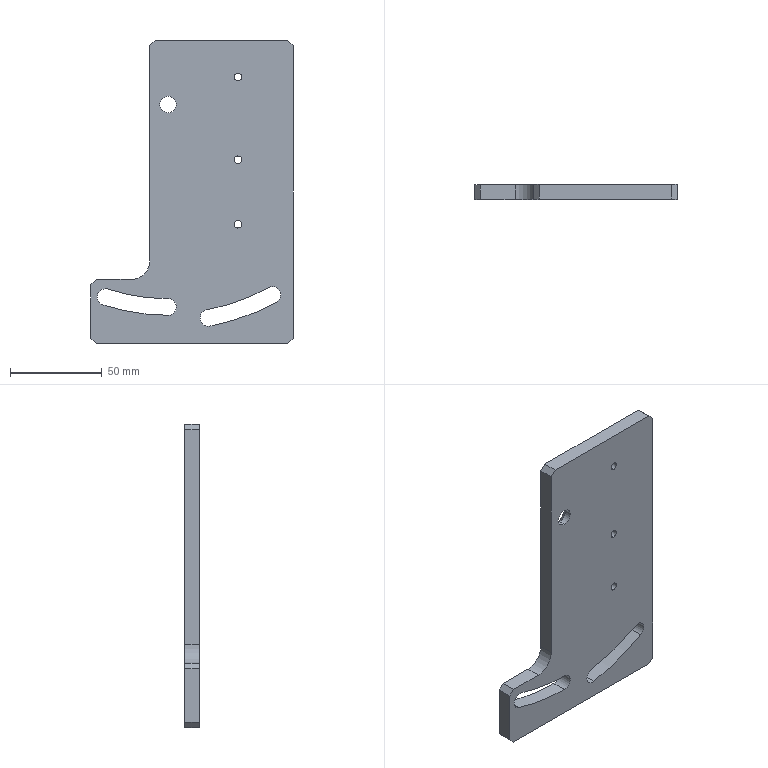Part | SolidWorks | features ICE 3, Chamfer 2, HoleWzd 2, Extrusion 1, Fillet 1 | 1 solid | 34 faces | box 110 x 8 x 165 mm | volume 104521 mm3 | cylinder 19 | plane 13 | cone 2 | commonest cylinder face diameters 9 x8 4.2 x6 20 x1 211 x1 227 x1 229 x1
STEP:
#1=CARTESIAN_POINT('',(25.,0.,60.4));
#2=VERTEX_POINT('',#1);
#3=CARTESIAN_POINT('',(25.,0.,64.6));
#4=VERTEX_POINT('',#3);
#5=CARTESIAN_POINT('',(25.,0.,62.5));
#6=DIRECTION('',(0.,1.,0.));
#7=DIRECTION('',(0.,0.,1.));
#8=AXIS2_PLACEMENT_3D('',#5,#6,#7);
#9=CIRCLE('',#8,2.1);
#10=EDGE_CURVE('',#2,#4,#9,.T.);
#11=ORIENTED_EDGE('',*,*,#10,.F.);
#12=CARTESIAN_POINT('',(25.,8.,60.4));
#13=VERTEX_POINT('',#12);
#14=CARTESIAN_POINT('',(25.,8.,60.4));
#15=DIRECTION('',(0.,1.,0.));
#16=VECTOR('',#15,1000.);
#17=LINE('',#14,#16);
#18=EDGE_CURVE('',#2,#13,#17,.T.);
#19=ORIENTED_EDGE('',*,*,#18,.T.);
#20=CARTESIAN_POINT('',(25.,8.,64.6));
#21=VERTEX_POINT('',#20);
#22=CARTESIAN_POINT('',(25.,8.,62.5));
#23=DIRECTION('',(0.,1.,0.));
#24=DIRECTION('',(0.,0.,1.));
#25=AXIS2_PLACEMENT_3D('',#22,#23,#24);
#26=CIRCLE('',#25,2.1);
#27=EDGE_CURVE('',#13,#21,#26,.T.);
#28=ORIENTED_EDGE('',*,*,#27,.T.);
#29=CARTESIAN_POINT('',(25.,8.,64.6));
#30=DIRECTION('',(0.,1.,0.));
#31=VECTOR('',#30,1000.);
#32=LINE('',#29,#31);
#33=EDGE_CURVE('',#4,#21,#32,.T.);
#34=ORIENTED_EDGE('',*,*,#33,.F.);
#35=EDGE_LOOP('',(#11,#19,#28,#34));
#36=FACE_OUTER_BOUND('',#35,.T.);
#37=CARTESIAN_POINT('',(25.,8.,62.5));
#38=DIRECTION('',(0.,1.,0.));
#39=DIRECTION('',(0.,0.,1.));
#40=AXIS2_PLACEMENT_3D('',#37,#38,#39);
#41=CYLINDRICAL_SURFACE('',#40,2.1);
#42=ADVANCED_FACE('',(#36),#41,.F.);
#43=CARTESIAN_POINT('',(25.,0.,15.4));
#44=VERTEX_POINT('',#43);
#45=CARTESIAN_POINT('',(25.,0.,19.6));
#46=VERTEX_POINT('',#45);
#47=CARTESIAN_POINT('',(25.,0.,17.5));
#48=DIRECTION('',(0.,1.,0.));
#49=DIRECTION('',(0.,0.,1.));
#50=AXIS2_PLACEMENT_3D('',#47,#48,#49);
#51=CIRCLE('',#50,2.1);
#52=EDGE_CURVE('',#44,#46,#51,.T.);
#53=ORIENTED_EDGE('',*,*,#52,.F.);
#54=CARTESIAN_POINT('',(25.,8.,15.4));
#55=VERTEX_POINT('',#54);
#56=CARTESIAN_POINT('',(25.,8.,15.4));
#57=DIRECTION('',(0.,1.,0.));
#58=VECTOR('',#57,1000.);
#59=LINE('',#56,#58);
#60=EDGE_CURVE('',#44,#55,#59,.T.);
#61=ORIENTED_EDGE('',*,*,#60,.T.);
#62=CARTESIAN_POINT('',(25.,8.,19.6));
#63=VERTEX_POINT('',#62);
#64=CARTESIAN_POINT('',(25.,8.,17.5));
#65=DIRECTION('',(0.,1.,0.));
#66=DIRECTION('',(0.,0.,1.));
#67=AXIS2_PLACEMENT_3D('',#64,#65,#66);
#68=CIRCLE('',#67,2.1);
#69=EDGE_CURVE('',#55,#63,#68,.T.);
#70=ORIENTED_EDGE('',*,*,#69,.T.);
#71=CARTESIAN_POINT('',(25.,8.,19.6));
#72=DIRECTION('',(0.,1.,0.));
#73=VECTOR('',#72,1000.);
#74=LINE('',#71,#73);
#75=EDGE_CURVE('',#46,#63,#74,.T.);
#76=ORIENTED_EDGE('',*,*,#75,.F.);
#77=EDGE_LOOP('',(#53,#61,#70,#76));
#78=FACE_OUTER_BOUND('',#77,.T.);
#79=CARTESIAN_POINT('',(25.,8.,17.5));
#80=DIRECTION('',(0.,1.,0.));
#81=DIRECTION('',(0.,0.,1.));
#82=AXIS2_PLACEMENT_3D('',#79,#80,#81);
#83=CYLINDRICAL_SURFACE('',#82,2.1);
#84=ADVANCED_FACE('',(#78),#83,.F.);
#85=CARTESIAN_POINT('',(25.,0.,-19.6));
#86=VERTEX_POINT('',#85);
#87=CARTESIAN_POINT('',(25.,0.,-15.4));
#88=VERTEX_POINT('',#87);
#89=CARTESIAN_POINT('',(25.,0.,-17.5));
#90=DIRECTION('',(0.,1.,0.));
#91=DIRECTION('',(0.,0.,1.));
#92=AXIS2_PLACEMENT_3D('',#89,#90,#91);
#93=CIRCLE('',#92,2.1);
#94=EDGE_CURVE('',#86,#88,#93,.T.);
#95=ORIENTED_EDGE('',*,*,#94,.F.);
#96=CARTESIAN_POINT('',(25.,8.,-19.6));
#97=VERTEX_POINT('',#96);
#98=CARTESIAN_POINT('',(25.,8.,-19.6));
#99=DIRECTION('',(0.,1.,0.));
#100=VECTOR('',#99,1000.);
#101=LINE('',#98,#100);
#102=EDGE_CURVE('',#86,#97,#101,.T.);
#103=ORIENTED_EDGE('',*,*,#102,.T.);
#104=CARTESIAN_POINT('',(25.,8.,-15.4));
#105=VERTEX_POINT('',#104);
#106=CARTESIAN_POINT('',(25.,8.,-17.5));
#107=DIRECTION('',(0.,1.,0.));
#108=DIRECTION('',(0.,0.,1.));
#109=AXIS2_PLACEMENT_3D('',#106,#107,#108);
#110=CIRCLE('',#109,2.1);
#111=EDGE_CURVE('',#97,#105,#110,.T.);
#112=ORIENTED_EDGE('',*,*,#111,.T.);
#113=CARTESIAN_POINT('',(25.,8.,-15.4));
#114=DIRECTION('',(0.,1.,0.));
#115=VECTOR('',#114,1000.);
#116=LINE('',#113,#115);
#117=EDGE_CURVE('',#88,#105,#116,.T.);
#118=ORIENTED_EDGE('',*,*,#117,.F.);
#119=EDGE_LOOP('',(#95,#103,#112,#118));
#120=FACE_OUTER_BOUND('',#119,.T.);
#121=CARTESIAN_POINT('',(25.,8.,-17.5));
#122=DIRECTION('',(0.,1.,0.));
#123=DIRECTION('',(0.,0.,1.));
#124=AXIS2_PLACEMENT_3D('',#121,#122,#123);
#125=CYLINDRICAL_SURFACE('',#124,2.1);
#126=ADVANCED_FACE('',(#120),#125,.F.);
#127=CARTESIAN_POINT('',(43.672,0.,-51.5));
#128=VERTEX_POINT('',#127);
#129=CARTESIAN_POINT('',(45.834,0.,-59.947));
#130=VERTEX_POINT('',#129);
#131=CARTESIAN_POINT('',(43.672,0.,-56.));
#132=DIRECTION('',(0.,1.,0.));
#133=DIRECTION('',(0.,0.,1.));
#134=AXIS2_PLACEMENT_3D('',#131,#132,#133);
#135=CIRCLE('',#134,4.5);
#136=EDGE_CURVE('',#128,#130,#135,.T.);
#137=ORIENTED_EDGE('',*,*,#136,.F.);
#138=CARTESIAN_POINT('',(43.672,8.,-51.5));
#139=VERTEX_POINT('',#138);
#140=CARTESIAN_POINT('',(43.672,0.,-51.5));
#141=DIRECTION('',(0.,1.,0.));
#142=VECTOR('',#141,1000.);
#143=LINE('',#140,#142);
#144=EDGE_CURVE('',#128,#139,#143,.T.);
#145=ORIENTED_EDGE('',*,*,#144,.T.);
#146=CARTESIAN_POINT('',(45.834,8.,-59.947));
#147=VERTEX_POINT('',#146);
#148=CARTESIAN_POINT('',(43.672,8.,-56.));
#149=DIRECTION('',(0.,1.,0.));
#150=DIRECTION('',(0.,0.,1.));
#151=AXIS2_PLACEMENT_3D('',#148,#149,#150);
#152=CIRCLE('',#151,4.5);
#153=EDGE_CURVE('',#139,#147,#152,.T.);
#154=ORIENTED_EDGE('',*,*,#153,.T.);
#155=CARTESIAN_POINT('',(45.834,0.,-59.947));
#156=DIRECTION('',(0.,1.,0.));
#157=VECTOR('',#156,1000.);
#158=LINE('',#155,#157);
#159=EDGE_CURVE('',#130,#147,#158,.T.);
#160=ORIENTED_EDGE('',*,*,#159,.F.);
#161=EDGE_LOOP('',(#137,#145,#154,#160));
#162=FACE_OUTER_BOUND('',#161,.T.);
#163=CARTESIAN_POINT('',(43.672,0.,-56.));
#164=DIRECTION('',(0.,1.,0.));
#165=DIRECTION('',(0.,0.,1.));
#166=AXIS2_PLACEMENT_3D('',#163,#164,#165);
#167=CYLINDRICAL_SURFACE('',#166,4.5);
#168=ADVANCED_FACE('',(#162),#167,.F.);
#169=CARTESIAN_POINT('',(-46.992,0.,-52.616));
#170=VERTEX_POINT('',#169);
#171=CARTESIAN_POINT('',(-45.601,0.,-52.836));
#172=VERTEX_POINT('',#171);
#173=CARTESIAN_POINT('',(-46.992,0.,-57.116));
#174=DIRECTION('',(0.,1.,0.));
#175=DIRECTION('',(0.,0.,1.));
#176=AXIS2_PLACEMENT_3D('',#173,#174,#175);
#177=CIRCLE('',#176,4.5);
#178=EDGE_CURVE('',#170,#172,#177,.T.);
#179=ORIENTED_EDGE('',*,*,#178,.F.);
#180=CARTESIAN_POINT('',(-46.992,8.,-52.616));
#181=VERTEX_POINT('',#180);
#182=CARTESIAN_POINT('',(-46.992,0.,-52.616));
#183=DIRECTION('',(0.,1.,0.));
#184=VECTOR('',#183,1000.);
#185=LINE('',#182,#184);
#186=EDGE_CURVE('',#170,#181,#185,.T.);
#187=ORIENTED_EDGE('',*,*,#186,.T.);
#188=CARTESIAN_POINT('',(-45.601,8.,-52.836));
#189=VERTEX_POINT('',#188);
#190=CARTESIAN_POINT('',(-46.992,8.,-57.116));
#191=DIRECTION('',(0.,1.,0.));
#192=DIRECTION('',(0.,0.,1.));
#193=AXIS2_PLACEMENT_3D('',#190,#191,#192);
#194=CIRCLE('',#193,4.5);
#195=EDGE_CURVE('',#181,#189,#194,.T.);
#196=ORIENTED_EDGE('',*,*,#195,.T.);
#197=CARTESIAN_POINT('',(-45.601,0.,-52.836));
#198=DIRECTION('',(0.,1.,0.));
#199=VECTOR('',#198,1000.);
#200=LINE('',#197,#199);
#201=EDGE_CURVE('',#172,#189,#200,.T.);
#202=ORIENTED_EDGE('',*,*,#201,.F.);
#203=EDGE_LOOP('',(#179,#187,#196,#202));
#204=FACE_OUTER_BOUND('',#203,.T.);
#205=CARTESIAN_POINT('',(-46.992,0.,-57.116));
#206=DIRECTION('',(0.,1.,0.));
#207=DIRECTION('',(0.,0.,1.));
#208=AXIS2_PLACEMENT_3D('',#205,#206,#207);
#209=CYLINDRICAL_SURFACE('',#208,4.5);
#210=ADVANCED_FACE('',(#204),#209,.F.);
#211=CARTESIAN_POINT('',(-13.,3.54,43.));
#212=VERTEX_POINT('',#211);
#213=CARTESIAN_POINT('',(-13.,3.54,52.));
#214=VERTEX_POINT('',#213);
#215=CARTESIAN_POINT('',(-13.,3.54,47.5));
#216=DIRECTION('',(0.,1.,0.));
#217=DIRECTION('',(0.,0.,1.));
#218=AXIS2_PLACEMENT_3D('',#215,#216,#217);
#219=CIRCLE('',#218,4.5);
#220=EDGE_CURVE('',#212,#214,#219,.T.);
#221=ORIENTED_EDGE('',*,*,#220,.F.);
#222=CARTESIAN_POINT('',(-13.,8.,38.54));
#223=VERTEX_POINT('',#222);
#224=CARTESIAN_POINT('',(-13.,8.,38.54));
#225=DIRECTION('',(0.,0.7071,-0.7071));
#226=VECTOR('',#225,1000.);
#227=LINE('',#224,#226);
#228=EDGE_CURVE('',#212,#223,#227,.T.);
#229=ORIENTED_EDGE('',*,*,#228,.T.);
#230=CARTESIAN_POINT('',(-13.,8.,56.46));
#231=VERTEX_POINT('',#230);
#232=CARTESIAN_POINT('',(-13.,8.,47.5));
#233=DIRECTION('',(0.,1.,0.));
#234=DIRECTION('',(0.,0.,1.));
#235=AXIS2_PLACEMENT_3D('',#232,#233,#234);
#236=CIRCLE('',#235,8.96);
#237=EDGE_CURVE('',#223,#231,#236,.T.);
#238=ORIENTED_EDGE('',*,*,#237,.T.);
#239=CARTESIAN_POINT('',(-13.,8.,56.46));
#240=DIRECTION('',(0.,0.7071,0.7071));
#241=VECTOR('',#240,1000.);
#242=LINE('',#239,#241);
#243=EDGE_CURVE('',#214,#231,#242,.T.);
#244=ORIENTED_EDGE('',*,*,#243,.F.);
#245=EDGE_LOOP('',(#221,#229,#238,#244));
#246=FACE_OUTER_BOUND('',#245,.T.);
#247=CARTESIAN_POINT('',(-13.,8.,47.5));
#248=DIRECTION('',(0.,1.,0.));
#249=DIRECTION('',(0.,0.,1.));
#250=AXIS2_PLACEMENT_3D('',#247,#248,#249);
#251=CONICAL_SURFACE('',#250,8.96,0.7854);
#252=ADVANCED_FACE('',(#246),#251,.F.);
#253=CARTESIAN_POINT('',(-13.,0.,43.));
#254=VERTEX_POINT('',#253);
#255=CARTESIAN_POINT('',(-13.,0.,52.));
#256=VERTEX_POINT('',#255);
#257=CARTESIAN_POINT('',(-13.,0.,47.5));
#258=DIRECTION('',(0.,1.,0.));
#259=DIRECTION('',(0.,0.,1.));
#260=AXIS2_PLACEMENT_3D('',#257,#258,#259);
#261=CIRCLE('',#260,4.5);
#262=EDGE_CURVE('',#254,#256,#261,.T.);
#263=ORIENTED_EDGE('',*,*,#262,.F.);
#264=CARTESIAN_POINT('',(-13.,8.,43.));
#265=DIRECTION('',(0.,1.,0.));
#266=VECTOR('',#265,1000.);
#267=LINE('',#264,#266);
#268=EDGE_CURVE('',#254,#212,#267,.T.);
#269=ORIENTED_EDGE('',*,*,#268,.T.);
#270=ORIENTED_EDGE('',*,*,#220,.T.);
#271=CARTESIAN_POINT('',(-13.,8.,52.));
#272=DIRECTION('',(0.,1.,0.));
#273=VECTOR('',#272,1000.);
#274=LINE('',#271,#273);
#275=EDGE_CURVE('',#256,#214,#274,.T.);
#276=ORIENTED_EDGE('',*,*,#275,.F.);
#277=EDGE_LOOP('',(#263,#269,#270,#276));
#278=FACE_OUTER_BOUND('',#277,.T.);
#279=CARTESIAN_POINT('',(-13.,8.,47.5));
#280=DIRECTION('',(0.,1.,0.));
#281=DIRECTION('',(0.,0.,1.));
#282=AXIS2_PLACEMENT_3D('',#279,#280,#281);
#283=CYLINDRICAL_SURFACE('',#282,4.5);
#284=ADVANCED_FACE('',(#278),#283,.F.);
#285=CARTESIAN_POINT('',(55.,8.,79.5));
#286=VERTEX_POINT('',#285);
#287=CARTESIAN_POINT('',(55.,8.,-79.5));
#288=VERTEX_POINT('',#287);
#289=CARTESIAN_POINT('',(55.,8.,-82.5));
#290=DIRECTION('',(0.,0.,-1.));
#291=VECTOR('',#290,1000.);
#292=LINE('',#289,#291);
#293=EDGE_CURVE('',#286,#288,#292,.T.);
#294=ORIENTED_EDGE('',*,*,#293,.F.);
#295=CARTESIAN_POINT('',(55.,0.,79.5));
#296=VERTEX_POINT('',#295);
#297=CARTESIAN_POINT('',(55.,8.,79.5));
#298=DIRECTION('',(0.,-1.,0.));
#299=VECTOR('',#298,1000.);
#300=LINE('',#297,#299);
#301=EDGE_CURVE('',#286,#296,#300,.T.);
#302=ORIENTED_EDGE('',*,*,#301,.T.);
#303=CARTESIAN_POINT('',(55.,0.,-79.5));
#304=VERTEX_POINT('',#303);
#305=CARTESIAN_POINT('',(55.,0.,-82.5));
#306=DIRECTION('',(0.,0.,-1.));
#307=VECTOR('',#306,1000.);
#308=LINE('',#305,#307);
#309=EDGE_CURVE('',#296,#304,#308,.T.);
#310=ORIENTED_EDGE('',*,*,#309,.T.);
#311=CARTESIAN_POINT('',(55.,8.,-79.5));
#312=DIRECTION('',(0.,1.,0.));
#313=VECTOR('',#312,1000.);
#314=LINE('',#311,#313);
#315=EDGE_CURVE('',#304,#288,#314,.T.);
#316=ORIENTED_EDGE('',*,*,#315,.T.);
#317=EDGE_LOOP('',(#294,#302,#310,#316));
#318=FACE_OUTER_BOUND('',#317,.T.);
#319=CARTESIAN_POINT('',(55.,8.,-82.5));
#320=DIRECTION('',(-1.,0.,0.));
#321=DIRECTION('',(0.,0.,1.));
#322=AXIS2_PLACEMENT_3D('',#319,#320,#321);
#323=PLANE('',#322);
#324=ADVANCED_FACE('',(#318),#323,.F.);
#325=CARTESIAN_POINT('',(52.,0.,-82.5));
#326=VERTEX_POINT('',#325);
#327=CARTESIAN_POINT('',(-52.,0.,-82.5));
#328=VERTEX_POINT('',#327);
#329=CARTESIAN_POINT('',(-55.,0.,-82.5));
#330=DIRECTION('',(-1.,0.,0.));
#331=VECTOR('',#330,1000.);
#332=LINE('',#329,#331);
#333=EDGE_CURVE('',#326,#328,#332,.T.);
#334=ORIENTED_EDGE('',*,*,#333,.T.);
#335=CARTESIAN_POINT('',(-52.,8.,-82.5));
#336=VERTEX_POINT('',#335);
#337=CARTESIAN_POINT('',(-52.,8.,-82.5));
#338=DIRECTION('',(0.,1.,0.));
#339=VECTOR('',#338,1000.);
#340=LINE('',#337,#339);
#341=EDGE_CURVE('',#328,#336,#340,.T.);
#342=ORIENTED_EDGE('',*,*,#341,.T.);
#343=CARTESIAN_POINT('',(52.,8.,-82.5));
#344=VERTEX_POINT('',#343);
#345=CARTESIAN_POINT('',(-55.,8.,-82.5));
#346=DIRECTION('',(-1.,0.,0.));
#347=VECTOR('',#346,1000.);
#348=LINE('',#345,#347);
#349=EDGE_CURVE('',#344,#336,#348,.T.);
#350=ORIENTED_EDGE('',*,*,#349,.F.);
#351=CARTESIAN_POINT('',(52.,8.,-82.5));
#352=DIRECTION('',(0.,-1.,0.));
#353=VECTOR('',#352,1000.);
#354=LINE('',#351,#353);
#355=EDGE_CURVE('',#344,#326,#354,.T.);
#356=ORIENTED_EDGE('',*,*,#355,.T.);
#357=EDGE_LOOP('',(#334,#342,#350,#356));
#358=FACE_OUTER_BOUND('',#357,.T.);
#359=CARTESIAN_POINT('',(-55.,8.,-82.5));
#360=DIRECTION('',(0.,0.,1.));
#361=DIRECTION('',(1.,0.,0.));
#362=AXIS2_PLACEMENT_3D('',#359,#360,#361);
#363=PLANE('',#362);
#364=ADVANCED_FACE('',(#358),#363,.F.);
#365=CARTESIAN_POINT('',(-55.,0.,-79.5));
#366=VERTEX_POINT('',#365);
#367=CARTESIAN_POINT('',(-55.,0.,-50.5));
#368=VERTEX_POINT('',#367);
#369=CARTESIAN_POINT('',(-55.,0.,-82.5));
#370=DIRECTION('',(0.,0.,1.));
#371=VECTOR('',#370,1000.);
#372=LINE('',#369,#371);
#373=EDGE_CURVE('',#366,#368,#372,.T.);
#374=ORIENTED_EDGE('',*,*,#373,.T.);
#375=CARTESIAN_POINT('',(-55.,8.,-50.5));
#376=VERTEX_POINT('',#375);
#377=CARTESIAN_POINT('',(-55.,8.,-50.5));
#378=DIRECTION('',(0.,1.,0.));
#379=VECTOR('',#378,1000.);
#380=LINE('',#377,#379);
#381=EDGE_CURVE('',#368,#376,#380,.T.);
#382=ORIENTED_EDGE('',*,*,#381,.T.);
#383=CARTESIAN_POINT('',(-55.,8.,-79.5));
#384=VERTEX_POINT('',#383);
#385=CARTESIAN_POINT('',(-55.,8.,-82.5));
#386=DIRECTION('',(0.,0.,1.));
#387=VECTOR('',#386,1000.);
#388=LINE('',#385,#387);
#389=EDGE_CURVE('',#384,#376,#388,.T.);
#390=ORIENTED_EDGE('',*,*,#389,.F.);
#391=CARTESIAN_POINT('',(-55.,8.,-79.5));
#392=DIRECTION('',(0.,-1.,0.));
#393=VECTOR('',#392,1000.);
#394=LINE('',#391,#393);
#395=EDGE_CURVE('',#384,#366,#394,.T.);
#396=ORIENTED_EDGE('',*,*,#395,.T.);
#397=EDGE_LOOP('',(#374,#382,#390,#396));
#398=FACE_OUTER_BOUND('',#397,.T.);
#399=CARTESIAN_POINT('',(-55.,8.,-82.5));
#400=DIRECTION('',(1.,0.,0.));
#401=DIRECTION('',(0.,0.,-1.));
#402=AXIS2_PLACEMENT_3D('',#399,#400,#401);
#403=PLANE('',#402);
#404=ADVANCED_FACE('',(#398),#403,.F.);
#405=CARTESIAN_POINT('',(-20.,0.,82.5));
#406=VERTEX_POINT('',#405);
#407=CARTESIAN_POINT('',(52.,0.,82.5));
#408=VERTEX_POINT('',#407);
#409=CARTESIAN_POINT('',(-55.,0.,82.5));
#410=DIRECTION('',(1.,0.,0.));
#411=VECTOR('',#410,1000.);
#412=LINE('',#409,#411);
#413=EDGE_CURVE('',#406,#408,#412,.T.);
#414=ORIENTED_EDGE('',*,*,#413,.T.);
#415=CARTESIAN_POINT('',(52.,8.,82.5));
#416=VERTEX_POINT('',#415);
#417=CARTESIAN_POINT('',(52.,8.,82.5));
#418=DIRECTION('',(0.,1.,0.));
#419=VECTOR('',#418,1000.);
#420=LINE('',#417,#419);
#421=EDGE_CURVE('',#408,#416,#420,.T.);
#422=ORIENTED_EDGE('',*,*,#421,.T.);
#423=CARTESIAN_POINT('',(-20.,8.,82.5));
#424=VERTEX_POINT('',#423);
#425=CARTESIAN_POINT('',(-55.,8.,82.5));
#426=DIRECTION('',(1.,0.,0.));
#427=VECTOR('',#426,1000.);
#428=LINE('',#425,#427);
#429=EDGE_CURVE('',#424,#416,#428,.T.);
#430=ORIENTED_EDGE('',*,*,#429,.F.);
#431=CARTESIAN_POINT('',(-20.,8.,82.5));
#432=DIRECTION('',(0.,-1.,0.));
#433=VECTOR('',#432,1000.);
#434=LINE('',#431,#433);
#435=EDGE_CURVE('',#424,#406,#434,.T.);
#436=ORIENTED_EDGE('',*,*,#435,.T.);
#437=EDGE_LOOP('',(#414,#422,#430,#436));
#438=FACE_OUTER_BOUND('',#437,.T.);
#439=CARTESIAN_POINT('',(-55.,8.,82.5));
#440=DIRECTION('',(0.,0.,-1.));
#441=DIRECTION('',(-1.,0.,0.));
#442=AXIS2_PLACEMENT_3D('',#439,#440,#441);
#443=PLANE('',#442);
#444=ADVANCED_FACE('',(#438),#443,.F.);
#445=CARTESIAN_POINT('',(25.,8.,62.5));
#446=DIRECTION('',(0.,1.,0.));
#447=DIRECTION('',(0.,0.,1.));
#448=AXIS2_PLACEMENT_3D('',#445,#446,#447);
#449=CIRCLE('',#448,2.1);
#450=EDGE_CURVE('',#21,#13,#449,.T.);
#451=ORIENTED_EDGE('',*,*,#450,.F.);
#452=ORIENTED_EDGE('',*,*,#27,.F.);
#453=EDGE_LOOP('',(#451,#452));
#454=FACE_BOUND('',#453,.T.);
#455=CARTESIAN_POINT('',(25.,8.,17.5));
#456=DIRECTION('',(0.,1.,0.));
#457=DIRECTION('',(0.,0.,1.));
#458=AXIS2_PLACEMENT_3D('',#455,#456,#457);
#459=CIRCLE('',#458,2.1);
#460=EDGE_CURVE('',#63,#55,#459,.T.);
#461=ORIENTED_EDGE('',*,*,#460,.F.);
#462=ORIENTED_EDGE('',*,*,#69,.F.);
#463=EDGE_LOOP('',(#461,#462));
#464=FACE_BOUND('',#463,.T.);
#465=CARTESIAN_POINT('',(25.,8.,-17.5));
#466=DIRECTION('',(0.,1.,0.));
#467=DIRECTION('',(0.,0.,1.));
#468=AXIS2_PLACEMENT_3D('',#465,#466,#467);
#469=CIRCLE('',#468,2.1);
#470=EDGE_CURVE('',#105,#97,#469,.T.);
#471=ORIENTED_EDGE('',*,*,#470,.F.);
#472=ORIENTED_EDGE('',*,*,#111,.F.);
#473=EDGE_LOOP('',(#471,#472));
#474=FACE_BOUND('',#473,.T.);
#475=CARTESIAN_POINT('',(41.511,8.,-52.053));
#476=VERTEX_POINT('',#475);
#477=CARTESIAN_POINT('',(43.672,8.,-56.));
#478=DIRECTION('',(0.,1.,0.));
#479=DIRECTION('',(0.,0.,1.));
#480=AXIS2_PLACEMENT_3D('',#477,#478,#479);
#481=CIRCLE('',#480,4.5);
#482=EDGE_CURVE('',#476,#139,#481,.T.);
#483=ORIENTED_EDGE('',*,*,#482,.F.);
#484=CARTESIAN_POINT('',(8.08,8.,-64.025));
#485=VERTEX_POINT('',#484);
#486=CARTESIAN_POINT('',(-13.,8.,47.5));
#487=DIRECTION('',(0.,-1.,0.));
#488=DIRECTION('',(0.,0.,1.));
#489=AXIS2_PLACEMENT_3D('',#486,#487,#488);
#490=CIRCLE('',#489,113.5);
#491=EDGE_CURVE('',#485,#476,#490,.T.);
#492=ORIENTED_EDGE('',*,*,#491,.F.);
#493=CARTESIAN_POINT('',(9.751,8.,-72.869));
#494=VERTEX_POINT('',#493);
#495=CARTESIAN_POINT('',(8.915,8.,-68.447));
#496=DIRECTION('',(0.,1.,0.));
#497=DIRECTION('',(0.,0.,1.));
#498=AXIS2_PLACEMENT_3D('',#495,#496,#497);
#499=CIRCLE('',#498,4.5);
#500=EDGE_CURVE('',#494,#485,#499,.T.);
#501=ORIENTED_EDGE('',*,*,#500,.F.);
#502=CARTESIAN_POINT('',(-13.,8.,47.5));
#503=DIRECTION('',(0.,1.,0.));
#504=DIRECTION('',(0.,0.,1.));
#505=AXIS2_PLACEMENT_3D('',#502,#503,#504);
#506=CIRCLE('',#505,122.5);
#507=EDGE_CURVE('',#147,#494,#506,.T.);
#508=ORIENTED_EDGE('',*,*,#507,.F.);
#509=ORIENTED_EDGE('',*,*,#153,.F.);
#510=EDGE_LOOP('',(#483,#492,#501,#508,#509));
#511=FACE_BOUND('',#510,.T.);
#512=CARTESIAN_POINT('',(-13.,8.,-58.));
#513=VERTEX_POINT('',#512);
#514=CARTESIAN_POINT('',(-13.,8.,-67.));
#515=VERTEX_POINT('',#514);
#516=CARTESIAN_POINT('',(-13.,8.,-62.5));
#517=DIRECTION('',(0.,1.,0.));
#518=DIRECTION('',(0.,0.,1.));
#519=AXIS2_PLACEMENT_3D('',#516,#517,#518);
#520=CIRCLE('',#519,4.5);
#521=EDGE_CURVE('',#513,#515,#520,.T.);
#522=ORIENTED_EDGE('',*,*,#521,.F.);
#523=CARTESIAN_POINT('',(-13.,8.,47.5));
#524=DIRECTION('',(0.,1.,0.));
#525=DIRECTION('',(0.,0.,1.));
#526=AXIS2_PLACEMENT_3D('',#523,#524,#525);
#527=CIRCLE('',#526,105.5);
#528=EDGE_CURVE('',#513,#189,#527,.T.);
#529=ORIENTED_EDGE('',*,*,#528,.T.);
#530=ORIENTED_EDGE('',*,*,#195,.F.);
#531=CARTESIAN_POINT('',(-48.382,8.,-61.396));
#532=VERTEX_POINT('',#531);
#533=CARTESIAN_POINT('',(-46.992,8.,-57.116));
#534=DIRECTION('',(0.,1.,0.));
#535=DIRECTION('',(0.,0.,1.));
#536=AXIS2_PLACEMENT_3D('',#533,#534,#535);
#537=CIRCLE('',#536,4.5);
#538=EDGE_CURVE('',#532,#181,#537,.T.);
#539=ORIENTED_EDGE('',*,*,#538,.F.);
#540=CARTESIAN_POINT('',(-13.,8.,47.5));
#541=DIRECTION('',(0.,1.,0.));
#542=DIRECTION('',(0.,0.,1.));
#543=AXIS2_PLACEMENT_3D('',#540,#541,#542);
#544=CIRCLE('',#543,114.5);
#545=EDGE_CURVE('',#515,#532,#544,.T.);
#546=ORIENTED_EDGE('',*,*,#545,.F.);
#547=EDGE_LOOP('',(#522,#529,#530,#539,#546));
#548=FACE_BOUND('',#547,.T.);
#549=CARTESIAN_POINT('',(-13.,8.,47.5));
#550=DIRECTION('',(0.,1.,0.));
#551=DIRECTION('',(0.,0.,1.));
#552=AXIS2_PLACEMENT_3D('',#549,#550,#551);
#553=CIRCLE('',#552,8.96);
#554=EDGE_CURVE('',#231,#223,#553,.T.);
#555=ORIENTED_EDGE('',*,*,#554,.F.);
#556=ORIENTED_EDGE('',*,*,#237,.F.);
#557=EDGE_LOOP('',(#555,#556));
#558=FACE_BOUND('',#557,.T.);
#559=ORIENTED_EDGE('',*,*,#429,.T.);
#560=CARTESIAN_POINT('',(67.25,8.,67.25));
#561=DIRECTION('',(0.7071,0.,-0.7071));
#562=VECTOR('',#561,1000.);
#563=LINE('',#560,#562);
#564=EDGE_CURVE('',#416,#286,#563,.T.);
#565=ORIENTED_EDGE('',*,*,#564,.T.);
#566=ORIENTED_EDGE('',*,*,#293,.T.);
#567=CARTESIAN_POINT('',(67.25,8.,-67.25));
#568=DIRECTION('',(-0.7071,0.,-0.7071));
#569=VECTOR('',#568,1000.);
#570=LINE('',#567,#569);
#571=EDGE_CURVE('',#288,#344,#570,.T.);
#572=ORIENTED_EDGE('',*,*,#571,.T.);
#573=ORIENTED_EDGE('',*,*,#349,.T.);
#574=CARTESIAN_POINT('',(-67.25,8.,-67.25));
#575=DIRECTION('',(-0.7071,0.,0.7071));
#576=VECTOR('',#575,1000.);
#577=LINE('',#574,#576);
#578=EDGE_CURVE('',#336,#384,#577,.T.);
#579=ORIENTED_EDGE('',*,*,#578,.T.);
#580=ORIENTED_EDGE('',*,*,#389,.T.);
#581=CARTESIAN_POINT('',(-52.,8.,-47.5));
#582=VERTEX_POINT('',#581);
#583=CARTESIAN_POINT('',(-2.25,8.,2.25));
#584=DIRECTION('',(0.7071,0.,0.7071));
#585=VECTOR('',#584,1000.);
#586=LINE('',#583,#585);
#587=EDGE_CURVE('',#376,#582,#586,.T.);
#588=ORIENTED_EDGE('',*,*,#587,.T.);
#589=CARTESIAN_POINT('',(-33.,8.,-47.5));
#590=VERTEX_POINT('',#589);
#591=CARTESIAN_POINT('',(-55.,8.,-47.5));
#592=DIRECTION('',(-1.,0.,0.));
#593=VECTOR('',#592,1000.);
#594=LINE('',#591,#593);
#595=EDGE_CURVE('',#590,#582,#594,.T.);
#596=ORIENTED_EDGE('',*,*,#595,.F.);
#597=CARTESIAN_POINT('',(-23.,8.,-37.5));
#598=VERTEX_POINT('',#597);
#599=CARTESIAN_POINT('',(-33.,8.,-37.5));
#600=DIRECTION('',(0.,-1.,0.));
#601=DIRECTION('',(0.,0.,1.));
#602=AXIS2_PLACEMENT_3D('',#599,#600,#601);
#603=CIRCLE('',#602,10.);
#604=EDGE_CURVE('',#590,#598,#603,.T.);
#605=ORIENTED_EDGE('',*,*,#604,.T.);
#606=CARTESIAN_POINT('',(-23.,8.,79.5));
#607=VERTEX_POINT('',#606);
#608=CARTESIAN_POINT('',(-23.,8.,82.5));
#609=DIRECTION('',(0.,0.,-1.));
#610=VECTOR('',#609,1000.);
#611=LINE('',#608,#610);
#612=EDGE_CURVE('',#607,#598,#611,.T.);
#613=ORIENTED_EDGE('',*,*,#612,.F.);
#614=CARTESIAN_POINT('',(-51.25,8.,51.25));
#615=DIRECTION('',(0.7071,0.,0.7071));
#616=VECTOR('',#615,1000.);
#617=LINE('',#614,#616);
#618=EDGE_CURVE('',#607,#424,#617,.T.);
#619=ORIENTED_EDGE('',*,*,#618,.T.);
#620=EDGE_LOOP('',(#559,#565,#566,#572,#573,#579,#580,#588,#596,#605,#613,#619));
#621=FACE_OUTER_BOUND('',#620,.T.);
#622=CARTESIAN_POINT('',(0.,8.,0.));
#623=DIRECTION('',(0.,1.,0.));
#624=DIRECTION('',(0.,0.,1.));
#625=AXIS2_PLACEMENT_3D('',#622,#623,#624);
#626=PLANE('',#625);
#627=ADVANCED_FACE('',(#454,#464,#474,#511,#548,#558,#621),#626,.T.);
#628=CARTESIAN_POINT('',(25.,0.,62.5));
#629=DIRECTION('',(0.,1.,0.));
#630=DIRECTION('',(0.,0.,1.));
#631=AXIS2_PLACEMENT_3D('',#628,#629,#630);
#632=CIRCLE('',#631,2.1);
#633=EDGE_CURVE('',#4,#2,#632,.T.);
#634=ORIENTED_EDGE('',*,*,#633,.T.);
#635=ORIENTED_EDGE('',*,*,#10,.T.);
#636=EDGE_LOOP('',(#634,#635));
#637=FACE_BOUND('',#636,.T.);
#638=CARTESIAN_POINT('',(25.,0.,17.5));
#639=DIRECTION('',(0.,1.,0.));
#640=DIRECTION('',(0.,0.,1.));
#641=AXIS2_PLACEMENT_3D('',#638,#639,#640);
#642=CIRCLE('',#641,2.1);
#643=EDGE_CURVE('',#46,#44,#642,.T.);
#644=ORIENTED_EDGE('',*,*,#643,.T.);
#645=ORIENTED_EDGE('',*,*,#52,.T.);
#646=EDGE_LOOP('',(#644,#645));
#647=FACE_BOUND('',#646,.T.);
#648=CARTESIAN_POINT('',(25.,0.,-17.5));
#649=DIRECTION('',(0.,1.,0.));
#650=DIRECTION('',(0.,0.,1.));
#651=AXIS2_PLACEMENT_3D('',#648,#649,#650);
#652=CIRCLE('',#651,2.1);
#653=EDGE_CURVE('',#88,#86,#652,.T.);
#654=ORIENTED_EDGE('',*,*,#653,.T.);
#655=ORIENTED_EDGE('',*,*,#94,.T.);
#656=EDGE_LOOP('',(#654,#655));
#657=FACE_BOUND('',#656,.T.);
#658=CARTESIAN_POINT('',(8.08,0.,-64.025));
#659=VERTEX_POINT('',#658);
#660=CARTESIAN_POINT('',(41.511,0.,-52.053));
#661=VERTEX_POINT('',#660);
#662=CARTESIAN_POINT('',(-13.,0.,47.5));
#663=DIRECTION('',(0.,-1.,0.));
#664=DIRECTION('',(0.,0.,1.));
#665=AXIS2_PLACEMENT_3D('',#662,#663,#664);
#666=CIRCLE('',#665,113.5);
#667=EDGE_CURVE('',#659,#661,#666,.T.);
#668=ORIENTED_EDGE('',*,*,#667,.T.);
#669=CARTESIAN_POINT('',(43.672,0.,-56.));
#670=DIRECTION('',(0.,1.,0.));
#671=DIRECTION('',(0.,0.,1.));
#672=AXIS2_PLACEMENT_3D('',#669,#670,#671);
#673=CIRCLE('',#672,4.5);
#674=EDGE_CURVE('',#661,#128,#673,.T.);
#675=ORIENTED_EDGE('',*,*,#674,.T.);
#676=ORIENTED_EDGE('',*,*,#136,.T.);
#677=CARTESIAN_POINT('',(9.751,0.,-72.869));
#678=VERTEX_POINT('',#677);
#679=CARTESIAN_POINT('',(-13.,0.,47.5));
#680=DIRECTION('',(0.,1.,0.));
#681=DIRECTION('',(0.,0.,1.));
#682=AXIS2_PLACEMENT_3D('',#679,#680,#681);
#683=CIRCLE('',#682,122.5);
#684=EDGE_CURVE('',#130,#678,#683,.T.);
#685=ORIENTED_EDGE('',*,*,#684,.T.);
#686=CARTESIAN_POINT('',(8.915,0.,-68.447));
#687=DIRECTION('',(0.,1.,0.));
#688=DIRECTION('',(0.,0.,1.));
#689=AXIS2_PLACEMENT_3D('',#686,#687,#688);
#690=CIRCLE('',#689,4.5);
#691=EDGE_CURVE('',#678,#659,#690,.T.);
#692=ORIENTED_EDGE('',*,*,#691,.T.);
#693=EDGE_LOOP('',(#668,#675,#676,#685,#692));
#694=FACE_BOUND('',#693,.T.);
#695=CARTESIAN_POINT('',(-13.,0.,-58.));
#696=VERTEX_POINT('',#695);
#697=CARTESIAN_POINT('',(-13.,0.,47.5));
#698=DIRECTION('',(0.,1.,0.));
#699=DIRECTION('',(0.,0.,1.));
#700=AXIS2_PLACEMENT_3D('',#697,#698,#699);
#701=CIRCLE('',#700,105.5);
#702=EDGE_CURVE('',#696,#172,#701,.T.);
#703=ORIENTED_EDGE('',*,*,#702,.F.);
#704=CARTESIAN_POINT('',(-13.,0.,-67.));
#705=VERTEX_POINT('',#704);
#706=CARTESIAN_POINT('',(-13.,0.,-62.5));
#707=DIRECTION('',(0.,1.,0.));
#708=DIRECTION('',(0.,0.,1.));
#709=AXIS2_PLACEMENT_3D('',#706,#707,#708);
#710=CIRCLE('',#709,4.5);
#711=EDGE_CURVE('',#696,#705,#710,.T.);
#712=ORIENTED_EDGE('',*,*,#711,.T.);
#713=CARTESIAN_POINT('',(-48.382,0.,-61.396));
#714=VERTEX_POINT('',#713);
#715=CARTESIAN_POINT('',(-13.,0.,47.5));
#716=DIRECTION('',(0.,1.,0.));
#717=DIRECTION('',(0.,0.,1.));
#718=AXIS2_PLACEMENT_3D('',#715,#716,#717);
#719=CIRCLE('',#718,114.5);
#720=EDGE_CURVE('',#705,#714,#719,.T.);
#721=ORIENTED_EDGE('',*,*,#720,.T.);
#722=CARTESIAN_POINT('',(-46.992,0.,-57.116));
#723=DIRECTION('',(0.,1.,0.));
#724=DIRECTION('',(0.,0.,1.));
#725=AXIS2_PLACEMENT_3D('',#722,#723,#724);
#726=CIRCLE('',#725,4.5);
#727=EDGE_CURVE('',#714,#170,#726,.T.);
#728=ORIENTED_EDGE('',*,*,#727,.T.);
#729=ORIENTED_EDGE('',*,*,#178,.T.);
#730=EDGE_LOOP('',(#703,#712,#721,#728,#729));
#731=FACE_BOUND('',#730,.T.);
#732=CARTESIAN_POINT('',(-13.,0.,47.5));
#733=DIRECTION('',(0.,1.,0.));
#734=DIRECTION('',(0.,0.,1.));
#735=AXIS2_PLACEMENT_3D('',#732,#733,#734);
#736=CIRCLE('',#735,4.5);
#737=EDGE_CURVE('',#256,#254,#736,.T.);
#738=ORIENTED_EDGE('',*,*,#737,.T.);
#739=ORIENTED_EDGE('',*,*,#262,.T.);
#740=EDGE_LOOP('',(#738,#739));
#741=FACE_BOUND('',#740,.T.);
#742=ORIENTED_EDGE('',*,*,#309,.F.);
#743=CARTESIAN_POINT('',(55.,0.,79.5));
#744=DIRECTION('',(-0.7071,0.,0.7071));
#745=VECTOR('',#744,1000.);
#746=LINE('',#743,#745);
#747=EDGE_CURVE('',#296,#408,#746,.T.);
#748=ORIENTED_EDGE('',*,*,#747,.T.);
#749=ORIENTED_EDGE('',*,*,#413,.F.);
#750=CARTESIAN_POINT('',(-23.,0.,79.5));
#751=VERTEX_POINT('',#750);
#752=CARTESIAN_POINT('',(-23.,0.,79.5));
#753=DIRECTION('',(-0.7071,0.,-0.7071));
#754=VECTOR('',#753,1000.);
#755=LINE('',#752,#754);
#756=EDGE_CURVE('',#406,#751,#755,.T.);
#757=ORIENTED_EDGE('',*,*,#756,.T.);
#758=CARTESIAN_POINT('',(-23.,0.,-37.5));
#759=VERTEX_POINT('',#758);
#760=CARTESIAN_POINT('',(-23.,0.,82.5));
#761=DIRECTION('',(0.,0.,-1.));
#762=VECTOR('',#761,1000.);
#763=LINE('',#760,#762);
#764=EDGE_CURVE('',#751,#759,#763,.T.);
#765=ORIENTED_EDGE('',*,*,#764,.T.);
#766=CARTESIAN_POINT('',(-33.,0.,-47.5));
#767=VERTEX_POINT('',#766);
#768=CARTESIAN_POINT('',(-33.,0.,-37.5));
#769=DIRECTION('',(0.,1.,0.));
#770=DIRECTION('',(0.,0.,1.));
#771=AXIS2_PLACEMENT_3D('',#768,#769,#770);
#772=CIRCLE('',#771,10.);
#773=EDGE_CURVE('',#759,#767,#772,.T.);
#774=ORIENTED_EDGE('',*,*,#773,.T.);
#775=CARTESIAN_POINT('',(-52.,0.,-47.5));
#776=VERTEX_POINT('',#775);
#777=CARTESIAN_POINT('',(-55.,0.,-47.5));
#778=DIRECTION('',(-1.,0.,0.));
#779=VECTOR('',#778,1000.);
#780=LINE('',#777,#779);
#781=EDGE_CURVE('',#767,#776,#780,.T.);
#782=ORIENTED_EDGE('',*,*,#781,.T.);
#783=CARTESIAN_POINT('',(-55.,0.,-50.5));
#784=DIRECTION('',(-0.7071,0.,-0.7071));
#785=VECTOR('',#784,1000.);
#786=LINE('',#783,#785);
#787=EDGE_CURVE('',#776,#368,#786,.T.);
#788=ORIENTED_EDGE('',*,*,#787,.T.);
#789=ORIENTED_EDGE('',*,*,#373,.F.);
#790=CARTESIAN_POINT('',(-55.,0.,-79.5));
#791=DIRECTION('',(0.7071,0.,-0.7071));
#792=VECTOR('',#791,1000.);
#793=LINE('',#790,#792);
#794=EDGE_CURVE('',#366,#328,#793,.T.);
#795=ORIENTED_EDGE('',*,*,#794,.T.);
#796=ORIENTED_EDGE('',*,*,#333,.F.);
#797=CARTESIAN_POINT('',(52.,0.,-82.5));
#798=DIRECTION('',(0.7071,0.,0.7071));
#799=VECTOR('',#798,1000.);
#800=LINE('',#797,#799);
#801=EDGE_CURVE('',#326,#304,#800,.T.);
#802=ORIENTED_EDGE('',*,*,#801,.T.);
#803=EDGE_LOOP('',(#742,#748,#749,#757,#765,#774,#782,#788,#789,#795,#796,#802));
#804=FACE_OUTER_BOUND('',#803,.T.);
#805=CARTESIAN_POINT('',(0.,0.,0.));
#806=DIRECTION('',(0.,1.,0.));
#807=DIRECTION('',(0.,0.,1.));
#808=AXIS2_PLACEMENT_3D('',#805,#806,#807);
#809=PLANE('',#808);
#810=ADVANCED_FACE('',(#637,#647,#657,#694,#731,#741,#804),#809,.F.);
#811=ORIENTED_EDGE('',*,*,#781,.F.);
#812=CARTESIAN_POINT('',(-33.,8.,-47.5));
#813=DIRECTION('',(0.,1.,0.));
#814=VECTOR('',#813,1000.);
#815=LINE('',#812,#814);
#816=EDGE_CURVE('',#767,#590,#815,.T.);
#817=ORIENTED_EDGE('',*,*,#816,.T.);
#818=ORIENTED_EDGE('',*,*,#595,.T.);
#819=CARTESIAN_POINT('',(-52.,0.,-47.5));
#820=DIRECTION('',(0.,-1.,0.));
#821=VECTOR('',#820,1000.);
#822=LINE('',#819,#821);
#823=EDGE_CURVE('',#582,#776,#822,.T.);
#824=ORIENTED_EDGE('',*,*,#823,.T.);
#825=EDGE_LOOP('',(#811,#817,#818,#824));
#826=FACE_OUTER_BOUND('',#825,.T.);
#827=CARTESIAN_POINT('',(-55.,0.,-47.5));
#828=DIRECTION('',(0.,0.,-1.));
#829=DIRECTION('',(-1.,0.,0.));
#830=AXIS2_PLACEMENT_3D('',#827,#828,#829);
#831=PLANE('',#830);
#832=ADVANCED_FACE('',(#826),#831,.F.);
#833=ORIENTED_EDGE('',*,*,#612,.T.);
#834=CARTESIAN_POINT('',(-23.,0.,-37.5));
#835=DIRECTION('',(0.,-1.,0.));
#836=VECTOR('',#835,1000.);
#837=LINE('',#834,#836);
#838=EDGE_CURVE('',#598,#759,#837,.T.);
#839=ORIENTED_EDGE('',*,*,#838,.T.);
#840=ORIENTED_EDGE('',*,*,#764,.F.);
#841=CARTESIAN_POINT('',(-23.,0.,79.5));
#842=DIRECTION('',(0.,1.,0.));
#843=VECTOR('',#842,1000.);
#844=LINE('',#841,#843);
#845=EDGE_CURVE('',#751,#607,#844,.T.);
#846=ORIENTED_EDGE('',*,*,#845,.T.);
#847=EDGE_LOOP('',(#833,#839,#840,#846));
#848=FACE_OUTER_BOUND('',#847,.T.);
#849=CARTESIAN_POINT('',(-23.,0.,82.5));
#850=DIRECTION('',(1.,0.,0.));
#851=DIRECTION('',(0.,0.,-1.));
#852=AXIS2_PLACEMENT_3D('',#849,#850,#851);
#853=PLANE('',#852);
#854=ADVANCED_FACE('',(#848),#853,.F.);
#855=ORIENTED_EDGE('',*,*,#268,.F.);
#856=ORIENTED_EDGE('',*,*,#737,.F.);
#857=ORIENTED_EDGE('',*,*,#275,.T.);
#858=CARTESIAN_POINT('',(-13.,3.54,47.5));
#859=DIRECTION('',(0.,1.,0.));
#860=DIRECTION('',(0.,0.,1.));
#861=AXIS2_PLACEMENT_3D('',#858,#859,#860);
#862=CIRCLE('',#861,4.5);
#863=EDGE_CURVE('',#214,#212,#862,.T.);
#864=ORIENTED_EDGE('',*,*,#863,.T.);
#865=EDGE_LOOP('',(#855,#856,#857,#864));
#866=FACE_OUTER_BOUND('',#865,.T.);
#867=CARTESIAN_POINT('',(-13.,8.,47.5));
#868=DIRECTION('',(0.,1.,0.));
#869=DIRECTION('',(0.,0.,1.));
#870=AXIS2_PLACEMENT_3D('',#867,#868,#869);
#871=CYLINDRICAL_SURFACE('',#870,4.5);
#872=ADVANCED_FACE('',(#866),#871,.F.);
#873=ORIENTED_EDGE('',*,*,#228,.F.);
#874=ORIENTED_EDGE('',*,*,#863,.F.);
#875=ORIENTED_EDGE('',*,*,#243,.T.);
#876=ORIENTED_EDGE('',*,*,#554,.T.);
#877=EDGE_LOOP('',(#873,#874,#875,#876));
#878=FACE_OUTER_BOUND('',#877,.T.);
#879=CARTESIAN_POINT('',(-13.,8.,47.5));
#880=DIRECTION('',(0.,1.,0.));
#881=DIRECTION('',(0.,0.,1.));
#882=AXIS2_PLACEMENT_3D('',#879,#880,#881);
#883=CONICAL_SURFACE('',#882,8.96,0.7854);
#884=ADVANCED_FACE('',(#878),#883,.F.);
#885=ORIENTED_EDGE('',*,*,#521,.T.);
#886=CARTESIAN_POINT('',(-13.,0.,-67.));
#887=DIRECTION('',(0.,1.,0.));
#888=VECTOR('',#887,1000.);
#889=LINE('',#886,#888);
#890=EDGE_CURVE('',#705,#515,#889,.T.);
#891=ORIENTED_EDGE('',*,*,#890,.F.);
#892=ORIENTED_EDGE('',*,*,#711,.F.);
#893=CARTESIAN_POINT('',(-13.,0.,-58.));
#894=DIRECTION('',(0.,1.,0.));
#895=VECTOR('',#894,1000.);
#896=LINE('',#893,#895);
#897=EDGE_CURVE('',#696,#513,#896,.T.);
#898=ORIENTED_EDGE('',*,*,#897,.T.);
#899=EDGE_LOOP('',(#885,#891,#892,#898));
#900=FACE_OUTER_BOUND('',#899,.T.);
#901=CARTESIAN_POINT('',(-13.,0.,-62.5));
#902=DIRECTION('',(0.,1.,0.));
#903=DIRECTION('',(0.,0.,1.));
#904=AXIS2_PLACEMENT_3D('',#901,#902,#903);
#905=CYLINDRICAL_SURFACE('',#904,4.5);
#906=ADVANCED_FACE('',(#900),#905,.F.);
#907=ORIENTED_EDGE('',*,*,#528,.F.);
#908=ORIENTED_EDGE('',*,*,#897,.F.);
#909=ORIENTED_EDGE('',*,*,#702,.T.);
#910=ORIENTED_EDGE('',*,*,#201,.T.);
#911=EDGE_LOOP('',(#907,#908,#909,#910));
#912=FACE_OUTER_BOUND('',#911,.T.);
#913=CARTESIAN_POINT('',(-13.,0.,47.5));
#914=DIRECTION('',(0.,1.,0.));
#915=DIRECTION('',(0.,0.,1.));
#916=AXIS2_PLACEMENT_3D('',#913,#914,#915);
#917=CYLINDRICAL_SURFACE('',#916,105.5);
#918=ADVANCED_FACE('',(#912),#917,.T.);
#919=ORIENTED_EDGE('',*,*,#186,.F.);
#920=ORIENTED_EDGE('',*,*,#727,.F.);
#921=CARTESIAN_POINT('',(-48.382,0.,-61.396));
#922=DIRECTION('',(0.,1.,0.));
#923=VECTOR('',#922,1000.);
#924=LINE('',#921,#923);
#925=EDGE_CURVE('',#714,#532,#924,.T.);
#926=ORIENTED_EDGE('',*,*,#925,.T.);
#927=ORIENTED_EDGE('',*,*,#538,.T.);
#928=EDGE_LOOP('',(#919,#920,#926,#927));
#929=FACE_OUTER_BOUND('',#928,.T.);
#930=CARTESIAN_POINT('',(-46.992,0.,-57.116));
#931=DIRECTION('',(0.,1.,0.));
#932=DIRECTION('',(0.,0.,1.));
#933=AXIS2_PLACEMENT_3D('',#930,#931,#932);
#934=CYLINDRICAL_SURFACE('',#933,4.5);
#935=ADVANCED_FACE('',(#929),#934,.F.);
#936=ORIENTED_EDGE('',*,*,#545,.T.);
#937=ORIENTED_EDGE('',*,*,#925,.F.);
#938=ORIENTED_EDGE('',*,*,#720,.F.);
#939=ORIENTED_EDGE('',*,*,#890,.T.);
#940=EDGE_LOOP('',(#936,#937,#938,#939));
#941=FACE_OUTER_BOUND('',#940,.T.);
#942=CARTESIAN_POINT('',(-13.,0.,47.5));
#943=DIRECTION('',(0.,1.,0.));
#944=DIRECTION('',(0.,0.,1.));
#945=AXIS2_PLACEMENT_3D('',#942,#943,#944);
#946=CYLINDRICAL_SURFACE('',#945,114.5);
#947=ADVANCED_FACE('',(#941),#946,.F.);
#948=ORIENTED_EDGE('',*,*,#144,.F.);
#949=ORIENTED_EDGE('',*,*,#674,.F.);
#950=CARTESIAN_POINT('',(41.511,0.,-52.053));
#951=DIRECTION('',(0.,1.,0.));
#952=VECTOR('',#951,1000.);
#953=LINE('',#950,#952);
#954=EDGE_CURVE('',#661,#476,#953,.T.);
#955=ORIENTED_EDGE('',*,*,#954,.T.);
#956=ORIENTED_EDGE('',*,*,#482,.T.);
#957=EDGE_LOOP('',(#948,#949,#955,#956));
#958=FACE_OUTER_BOUND('',#957,.T.);
#959=CARTESIAN_POINT('',(43.672,0.,-56.));
#960=DIRECTION('',(0.,1.,0.));
#961=DIRECTION('',(0.,0.,1.));
#962=AXIS2_PLACEMENT_3D('',#959,#960,#961);
#963=CYLINDRICAL_SURFACE('',#962,4.5);
#964=ADVANCED_FACE('',(#958),#963,.F.);
#965=ORIENTED_EDGE('',*,*,#491,.T.);
#966=ORIENTED_EDGE('',*,*,#954,.F.);
#967=ORIENTED_EDGE('',*,*,#667,.F.);
#968=CARTESIAN_POINT('',(8.08,0.,-64.025));
#969=DIRECTION('',(0.,1.,0.));
#970=VECTOR('',#969,1000.);
#971=LINE('',#968,#970);
#972=EDGE_CURVE('',#659,#485,#971,.T.);
#973=ORIENTED_EDGE('',*,*,#972,.T.);
#974=EDGE_LOOP('',(#965,#966,#967,#973));
#975=FACE_OUTER_BOUND('',#974,.T.);
#976=CARTESIAN_POINT('',(-13.,0.,47.5));
#977=DIRECTION('',(0.,1.,0.));
#978=DIRECTION('',(0.,0.,1.));
#979=AXIS2_PLACEMENT_3D('',#976,#977,#978);
#980=CYLINDRICAL_SURFACE('',#979,113.5);
#981=ADVANCED_FACE('',(#975),#980,.T.);
#982=ORIENTED_EDGE('',*,*,#500,.T.);
#983=ORIENTED_EDGE('',*,*,#972,.F.);
#984=ORIENTED_EDGE('',*,*,#691,.F.);
#985=CARTESIAN_POINT('',(9.751,0.,-72.869));
#986=DIRECTION('',(0.,1.,0.));
#987=VECTOR('',#986,1000.);
#988=LINE('',#985,#987);
#989=EDGE_CURVE('',#678,#494,#988,.T.);
#990=ORIENTED_EDGE('',*,*,#989,.T.);
#991=EDGE_LOOP('',(#982,#983,#984,#990));
#992=FACE_OUTER_BOUND('',#991,.T.);
#993=CARTESIAN_POINT('',(8.915,0.,-68.447));
#994=DIRECTION('',(0.,1.,0.));
#995=DIRECTION('',(0.,0.,1.));
#996=AXIS2_PLACEMENT_3D('',#993,#994,#995);
#997=CYLINDRICAL_SURFACE('',#996,4.5);
#998=ADVANCED_FACE('',(#992),#997,.F.);
#999=ORIENTED_EDGE('',*,*,#507,.T.);
#1000=ORIENTED_EDGE('',*,*,#989,.F.);
#1001=ORIENTED_EDGE('',*,*,#684,.F.);
#1002=ORIENTED_EDGE('',*,*,#159,.T.);
#1003=EDGE_LOOP('',(#999,#1000,#1001,#1002));
#1004=FACE_OUTER_BOUND('',#1003,.T.);
#1005=CARTESIAN_POINT('',(-13.,0.,47.5));
#1006=DIRECTION('',(0.,1.,0.));
#1007=DIRECTION('',(0.,0.,1.));
#1008=AXIS2_PLACEMENT_3D('',#1005,#1006,#1007);
#1009=CYLINDRICAL_SURFACE('',#1008,122.5);
#1010=ADVANCED_FACE('',(#1004),#1009,.F.);
#1011=ORIENTED_EDGE('',*,*,#564,.F.);
#1012=ORIENTED_EDGE('',*,*,#421,.F.);
#1013=ORIENTED_EDGE('',*,*,#747,.F.);
#1014=ORIENTED_EDGE('',*,*,#301,.F.);
#1015=EDGE_LOOP('',(#1011,#1012,#1013,#1014));
#1016=FACE_OUTER_BOUND('',#1015,.T.);
#1017=CARTESIAN_POINT('',(55.,8.,79.5));
#1018=DIRECTION('',(-0.7071,0.,-0.7071));
#1019=DIRECTION('',(0.,-1.,0.));
#1020=AXIS2_PLACEMENT_3D('',#1017,#1018,#1019);
#1021=PLANE('',#1020);
#1022=ADVANCED_FACE('',(#1016),#1021,.F.);
#1023=ORIENTED_EDGE('',*,*,#756,.F.);
#1024=ORIENTED_EDGE('',*,*,#435,.F.);
#1025=ORIENTED_EDGE('',*,*,#618,.F.);
#1026=ORIENTED_EDGE('',*,*,#845,.F.);
#1027=EDGE_LOOP('',(#1023,#1024,#1025,#1026));
#1028=FACE_OUTER_BOUND('',#1027,.T.);
#1029=CARTESIAN_POINT('',(-23.,0.,79.5));
#1030=DIRECTION('',(0.7071,0.,-0.7071));
#1031=DIRECTION('',(0.,1.,0.));
#1032=AXIS2_PLACEMENT_3D('',#1029,#1030,#1031);
#1033=PLANE('',#1032);
#1034=ADVANCED_FACE('',(#1028),#1033,.F.);
#1035=ORIENTED_EDGE('',*,*,#787,.F.);
#1036=ORIENTED_EDGE('',*,*,#823,.F.);
#1037=ORIENTED_EDGE('',*,*,#587,.F.);
#1038=ORIENTED_EDGE('',*,*,#381,.F.);
#1039=EDGE_LOOP('',(#1035,#1036,#1037,#1038));
#1040=FACE_OUTER_BOUND('',#1039,.T.);
#1041=CARTESIAN_POINT('',(-55.,8.,-50.5));
#1042=DIRECTION('',(0.7071,0.,-0.7071));
#1043=DIRECTION('',(0.,1.,0.));
#1044=AXIS2_PLACEMENT_3D('',#1041,#1042,#1043);
#1045=PLANE('',#1044);
#1046=ADVANCED_FACE('',(#1040),#1045,.F.);
#1047=ORIENTED_EDGE('',*,*,#578,.F.);
#1048=ORIENTED_EDGE('',*,*,#341,.F.);
#1049=ORIENTED_EDGE('',*,*,#794,.F.);
#1050=ORIENTED_EDGE('',*,*,#395,.F.);
#1051=EDGE_LOOP('',(#1047,#1048,#1049,#1050));
#1052=FACE_OUTER_BOUND('',#1051,.T.);
#1053=CARTESIAN_POINT('',(-55.,8.,-79.5));
#1054=DIRECTION('',(0.7071,0.,0.7071));
#1055=DIRECTION('',(0.,-1.,0.));
#1056=AXIS2_PLACEMENT_3D('',#1053,#1054,#1055);
#1057=PLANE('',#1056);
#1058=ADVANCED_FACE('',(#1052),#1057,.F.);
#1059=ORIENTED_EDGE('',*,*,#571,.F.);
#1060=ORIENTED_EDGE('',*,*,#315,.F.);
#1061=ORIENTED_EDGE('',*,*,#801,.F.);
#1062=ORIENTED_EDGE('',*,*,#355,.F.);
#1063=EDGE_LOOP('',(#1059,#1060,#1061,#1062));
#1064=FACE_OUTER_BOUND('',#1063,.T.);
#1065=CARTESIAN_POINT('',(52.,8.,-82.5));
#1066=DIRECTION('',(-0.7071,0.,0.7071));
#1067=DIRECTION('',(0.,-1.,0.));
#1068=AXIS2_PLACEMENT_3D('',#1065,#1066,#1067);
#1069=PLANE('',#1068);
#1070=ADVANCED_FACE('',(#1064),#1069,.F.);
#1071=ORIENTED_EDGE('',*,*,#102,.F.);
#1072=ORIENTED_EDGE('',*,*,#653,.F.);
#1073=ORIENTED_EDGE('',*,*,#117,.T.);
#1074=ORIENTED_EDGE('',*,*,#470,.T.);
#1075=EDGE_LOOP('',(#1071,#1072,#1073,#1074));
#1076=FACE_OUTER_BOUND('',#1075,.T.);
#1077=CARTESIAN_POINT('',(25.,8.,-17.5));
#1078=DIRECTION('',(0.,1.,0.));
#1079=DIRECTION('',(0.,0.,1.));
#1080=AXIS2_PLACEMENT_3D('',#1077,#1078,#1079);
#1081=CYLINDRICAL_SURFACE('',#1080,2.1);
#1082=ADVANCED_FACE('',(#1076),#1081,.F.);
#1083=ORIENTED_EDGE('',*,*,#60,.F.);
#1084=ORIENTED_EDGE('',*,*,#643,.F.);
#1085=ORIENTED_EDGE('',*,*,#75,.T.);
#1086=ORIENTED_EDGE('',*,*,#460,.T.);
#1087=EDGE_LOOP('',(#1083,#1084,#1085,#1086));
#1088=FACE_OUTER_BOUND('',#1087,.T.);
#1089=CARTESIAN_POINT('',(25.,8.,17.5));
#1090=DIRECTION('',(0.,1.,0.));
#1091=DIRECTION('',(0.,0.,1.));
#1092=AXIS2_PLACEMENT_3D('',#1089,#1090,#1091);
#1093=CYLINDRICAL_SURFACE('',#1092,2.1);
#1094=ADVANCED_FACE('',(#1088),#1093,.F.);
#1095=ORIENTED_EDGE('',*,*,#18,.F.);
#1096=ORIENTED_EDGE('',*,*,#633,.F.);
#1097=ORIENTED_EDGE('',*,*,#33,.T.);
#1098=ORIENTED_EDGE('',*,*,#450,.T.);
#1099=EDGE_LOOP('',(#1095,#1096,#1097,#1098));
#1100=FACE_OUTER_BOUND('',#1099,.T.);
#1101=CARTESIAN_POINT('',(25.,8.,62.5));
#1102=DIRECTION('',(0.,1.,0.));
#1103=DIRECTION('',(0.,0.,1.));
#1104=AXIS2_PLACEMENT_3D('',#1101,#1102,#1103);
#1105=CYLINDRICAL_SURFACE('',#1104,2.1);
#1106=ADVANCED_FACE('',(#1100),#1105,.F.);
#1107=ORIENTED_EDGE('',*,*,#773,.F.);
#1108=ORIENTED_EDGE('',*,*,#838,.F.);
#1109=ORIENTED_EDGE('',*,*,#604,.F.);
#1110=ORIENTED_EDGE('',*,*,#816,.F.);
#1111=EDGE_LOOP('',(#1107,#1108,#1109,#1110));
#1112=FACE_OUTER_BOUND('',#1111,.T.);
#1113=CARTESIAN_POINT('',(-33.,0.,-37.5));
#1114=DIRECTION('',(0.,-1.,0.));
#1115=DIRECTION('',(0.,0.,-1.));
#1116=AXIS2_PLACEMENT_3D('',#1113,#1114,#1115);
#1117=CYLINDRICAL_SURFACE('',#1116,10.);
#1118=ADVANCED_FACE('',(#1112),#1117,.F.);
#1119=CLOSED_SHELL('',(#42,#84,#126,#168,#210,#252,#284,#324,#364,#404,#444,#627,#810,#832,#854,#872,#884,#906,#918,#935,#947,#964,#981,#998,#1010,#1022,#1034,#1046,#1058,#1070,#1082,#1094,#1106,#1118));
#1120=MANIFOLD_SOLID_BREP('',#1119);
#1121=CARTESIAN_POINT('',(0.,0.,0.));
#1122=DIRECTION('',(0.,0.,1.));
#1123=DIRECTION('',(1.,0.,0.));
#1124=AXIS2_PLACEMENT_3D('',#1121,#1122,#1123);
#1125=(LENGTH_UNIT()NAMED_UNIT(*)SI_UNIT(.MILLI.,.METRE.));
#1126=UNCERTAINTY_MEASURE_WITH_UNIT(LENGTH_MEASURE(0.00001),#1125,'','');
#1127=(NAMED_UNIT(*)PLANE_ANGLE_UNIT()SI_UNIT($,.RADIAN.));
#1128=(NAMED_UNIT(*)SI_UNIT($,.STERADIAN.)SOLID_ANGLE_UNIT());
#1129=(GEOMETRIC_REPRESENTATION_CONTEXT(3)GLOBAL_UNCERTAINTY_ASSIGNED_CONTEXT((#1126))GLOBAL_UNIT_ASSIGNED_CONTEXT((#1125,#1127,#1128))REPRESENTATION_CONTEXT('',''));
#1130=ADVANCED_BREP_SHAPE_REPRESENTATION('',(#1120,#1124),#1129);